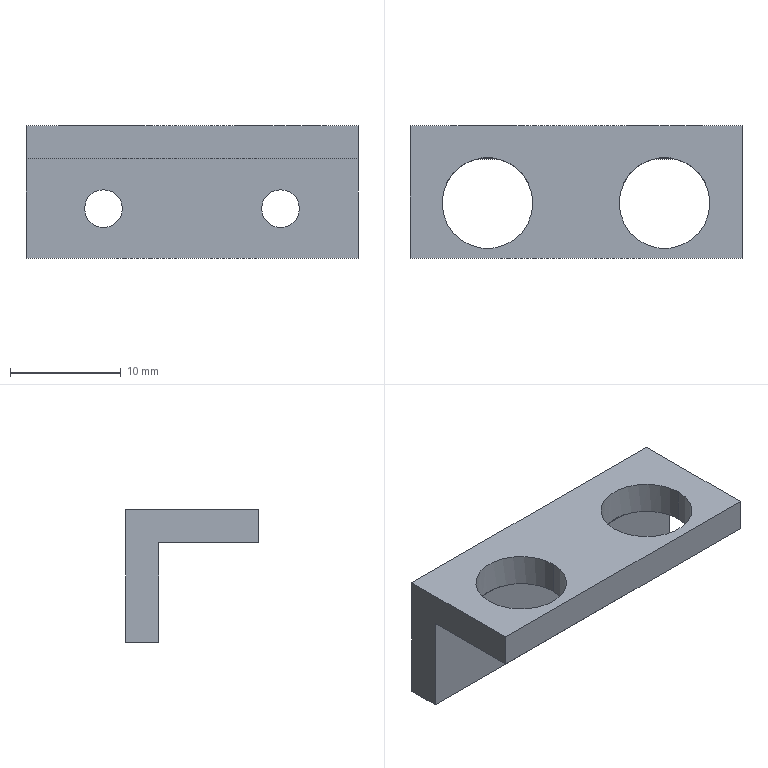NC program | NX | posted with a generic post | part box 30 x 12 x 12 mm
Lines 28 to 883 of 1871:
(ZLEVEL_PROFILE_1_1 , TOOL : D3R0.5)
N48 T07 M6
N50 G54
N52 G17 G0 G90 X-7.408 Y2.838 B0. C0. S7500 M3
N54 G43 Z30. H7
N56 Z0.929
N58 G94 G1 Z-0.071 F1000.
N60 X-7.74 Y3.413
N62 G3 X-7.999 Y3.563 R0.3
N64 X-10.062 Y1.5 R2.063 F2500.
N66 X-7.999 Y3.563 R-2.063
N68 G1 X-8.118 Y3.559 Z-0.073
N70 X-8.237 Y3.548 Z-0.075
N72 X-8.354 Y3.53 Z-0.077
N74 X-8.47 Y3.503 Z-0.079
N76 X-8.585 Y3.473 Z-0.081
N78 X-8.697 Y3.432 Z-0.083
N80 X-8.806 Y3.387 Z-0.085
N82 X-8.914 Y3.338 Z-0.087
N84 X-9.016 Y3.278 Z-0.089
N86 X-9.118 Y3.216 Z-0.092
N88 X-9.213 Y3.146 Z-0.094
N90 X-9.305 Y3.072 Z-0.096
N92 X-9.394 Y2.995 Z-0.098
N94 X-9.475 Y2.909 Z-0.1
N96 X-9.552 Y2.82 Z-0.102
N98 X-9.625 Y2.728 Z-0.104
N100 X-9.69 Y2.63 Z-0.106
N102 X-9.754 Y2.531 Z-0.108
N104 X-9.806 Y2.426 Z-0.11
N106 X-9.856 Y2.32 Z-0.112
N108 X-9.899 Y2.211 Z-0.114
N110 X-9.934 Y2.099 Z-0.116
N112 X-9.965 Y1.986 Z-0.119
N114 X-9.987 Y1.872 Z-0.121
N116 X-10.003 Y1.756 Z-0.123
N118 X-10.015 Y1.64 Z-0.125
N120 Y1.523 Z-0.127
N122 X-10.013 Y1.407 Z-0.129
N124 X-10.002 Y1.291 Z-0.131
N126 X-9.984 Y1.176 Z-0.133
N128 X-9.963 Y1.062 Z-0.135
N130 X-9.93 Y0.951 Z-0.137
N132 X-9.893 Y0.841 Z-0.139
N134 X-9.848 Y0.734 Z-0.141
N136 G3 X-7.999 Y3.501 R-2.001
N138 G1 X-8.118 Y3.497 Z-0.144
N140 X-8.237 Y3.486 Z-0.146
N142 X-8.354 Y3.467 Z-0.148
N144 X-8.47 Y3.439 Z-0.15
N146 X-8.585 Y3.409 Z-0.152
N148 X-8.696 Y3.366 Z-0.154
N150 X-8.805 Y3.321 Z-0.156
N152 X-8.912 Y3.268 Z-0.158
N154 X-9.014 Y3.208 Z-0.16
N156 X-9.114 Y3.146 Z-0.162
N158 X-9.207 Y3.073 Z-0.164
N160 X-9.298 Y2.997 Z-0.166
N162 X-9.384 Y2.916 Z-0.168
N164 X-9.464 Y2.829 Z-0.171
N166 X-9.541 Y2.741 Z-0.173
N168 X-9.609 Y2.644 Z-0.175
N170 X-9.673 Y2.546 Z-0.177
N172 X-9.731 Y2.444 Z-0.179
N174 X-9.781 Y2.338 Z-0.181
N176 X-9.828 Y2.23 Z-0.183
N178 X-9.865 Y2.119 Z-0.185
N180 X-9.897 Y2.007 Z-0.187
N182 X-9.923 Y1.893 Z-0.189
N184 X-9.94 Y1.777 Z-0.191
N186 X-9.953 Y1.661 Z-0.193
N188 X-9.955 Y1.544 Z-0.195
N190 X-9.953 Y1.428 Z-0.198
N192 X-9.944 Y1.312 Z-0.2
N194 X-9.927 Y1.197 Z-0.202
N196 X-9.904 Y1.083 Z-0.204
N198 X-9.874 Y0.971 Z-0.206
N200 X-9.837 Y0.861 Z-0.208
N202 X-9.794 Y0.754 Z-0.21
N204 X-9.744 Y0.649 Z-0.212
N206 G3 X-7.999 Y3.441 R-1.941
N208 G1 X-8.118 Y3.435 Z-0.214
N210 X-8.237 Y3.422 Z-0.216
N212 X-8.354 Y3.402 Z-0.218
N214 X-8.469 Y3.375 Z-0.22
N216 X-8.583 Y3.34 Z-0.223
N218 X-8.694 Y3.299 Z-0.225
N220 X-8.802 Y3.251 Z-0.227
N222 X-8.907 Y3.197 Z-0.229
N224 X-9.008 Y3.136 Z-0.231
N226 X-9.106 Y3.07 Z-0.233
N228 X-9.198 Y2.997 Z-0.235
N230 X-9.287 Y2.919 Z-0.237
N232 X-9.37 Y2.836 Z-0.239
N234 X-9.448 Y2.748 Z-0.241
N236 X-9.52 Y2.656 Z-0.243
N238 X-9.586 Y2.559 Z-0.245
N240 X-9.646 Y2.459 Z-0.247
N242 X-9.7 Y2.355 Z-0.25
N244 X-9.748 Y2.249 Z-0.252
N246 X-9.788 Y2.139 Z-0.254
N248 X-9.822 Y2.028 Z-0.256
N250 X-9.849 Y1.914 Z-0.258
N252 X-9.869 Y1.8 Z-0.26
N254 X-9.882 Y1.684 Z-0.262
N256 X-9.888 Y1.569 Z-0.264
N258 X-9.886 Y1.453 Z-0.266
N260 X-9.878 Y1.337 Z-0.268
N262 X-9.862 Y1.223 Z-0.27
N264 X-9.839 Y1.109 Z-0.272
N266 X-9.81 Y0.998 Z-0.275
N268 X-9.774 Y0.888 Z-0.277
N270 X-9.731 Y0.781 Z-0.279
N272 X-9.682 Y0.678 Z-0.281
N274 X-9.626 Y0.577 Z-0.283
N276 G3 X-7.999 Y3.37 R-1.87
N278 G1 X-8.118 Y3.364 Z-0.285
N280 X-8.237 Y3.351 Z-0.287
N282 X-8.353 Y3.33 Z-0.289
N284 X-8.469 Y3.302 Z-0.291
N286 X-8.582 Y3.266 Z-0.293
N288 X-8.692 Y3.224 Z-0.295
N290 X-8.8 Y3.174 Z-0.297
N292 X-8.904 Y3.118 Z-0.299
N294 X-9.004 Y3.056 Z-0.302
N296 X-9.1 Y2.987 Z-0.304
N298 X-9.191 Y2.912 Z-0.306
N300 X-9.277 Y2.832 Z-0.308
N302 X-9.357 Y2.747 Z-0.31
N304 X-9.432 Y2.656 Z-0.312
N306 X-9.501 Y2.562 Z-0.314
N308 X-9.564 Y2.463 Z-0.316
N310 X-9.621 Y2.36 Z-0.318
N312 X-9.67 Y2.254 Z-0.32
N314 X-9.713 Y2.146 Z-0.322
N316 X-9.748 Y2.035 Z-0.324
N318 X-9.777 Y1.922 Z-0.327
N320 X-9.798 Y1.808 Z-0.329
N322 X-9.812 Y1.692 Z-0.331
N324 X-9.819 Y1.576 Z-0.333
N326 X-9.818 Y1.461 Z-0.335
N328 X-9.809 Y1.345 Z-0.337
N330 X-9.794 Y1.231 Z-0.339
N332 X-9.771 Y1.117 Z-0.341
N334 X-9.741 Y1.006 Z-0.343
N336 X-9.704 Y0.897 Z-0.345
N338 X-9.66 Y0.79 Z-0.347
N340 X-9.61 Y0.687 Z-0.349
N342 X-9.553 Y0.587 Z-0.351
N344 X-9.49 Y0.491 Z-0.354
N346 G3 X-7.999 Y3.299 R-1.799
N348 G1 X-8.118 Y3.293 Z-0.356
N350 X-8.237 Y3.28 Z-0.358
N352 X-8.353 Y3.258 Z-0.36
N354 X-8.468 Y3.229 Z-0.362
N356 X-8.581 Y3.192 Z-0.364
N358 X-8.691 Y3.148 Z-0.366
N360 X-8.797 Y3.097 Z-0.368
N362 X-8.9 Y3.039 Z-0.37
N364 X-8.999 Y2.974 Z-0.372
N366 X-9.093 Y2.903 Z-0.374
N368 X-9.182 Y2.826 Z-0.376
N370 X-9.266 Y2.743 Z-0.379
N372 X-9.344 Y2.656 Z-0.381
N374 X-9.416 Y2.563 Z-0.383
N376 X-9.481 Y2.466 Z-0.385
N378 X-9.54 Y2.365 Z-0.387
N380 X-9.592 Y2.26 Z-0.389
N382 X-9.637 Y2.152 Z-0.391
N384 X-9.674 Y2.042 Z-0.393
N386 X-9.705 Y1.929 Z-0.395
N388 X-9.727 Y1.815 Z-0.397
N390 X-9.742 Y1.7 Z-0.399
N392 X-9.749 Y1.584 Z-0.401
N394 Y1.468 Z-0.403
N396 X-9.741 Y1.353 Z-0.406
N398 X-9.726 Y1.238 Z-0.408
N400 X-9.702 Y1.125 Z-0.41
N402 X-9.672 Y1.014 Z-0.412
N404 X-9.634 Y0.905 Z-0.414
N406 X-9.589 Y0.799 Z-0.416
N408 X-9.538 Y0.696 Z-0.418
N410 X-9.479 Y0.597 Z-0.42
N412 X-9.415 Y0.503 Z-0.422
N414 X-9.344 Y0.413 Z-0.424
N416 G3 X-7.999 Y3.229 R-1.729
N418 G1 X-8.118 Y3.222 Z-0.426
N420 X-8.236 Y3.208 Z-0.428
N422 X-8.353 Y3.186 Z-0.431
N424 X-8.468 Y3.155 Z-0.433
N426 X-8.58 Y3.117 Z-0.435
N428 X-8.689 Y3.072 Z-0.437
N430 X-8.795 Y3.019 Z-0.439
N432 X-8.896 Y2.959 Z-0.441
N434 X-8.993 Y2.892 Z-0.443
N436 X-9.086 Y2.818 Z-0.445
N438 X-9.172 Y2.739 Z-0.447
N440 X-9.254 Y2.654 Z-0.449
N442 X-9.328 Y2.564 Z-0.451
N444 X-9.397 Y2.468 Z-0.453
N446 X-9.458 Y2.369 Z-0.455
N448 X-9.513 Y2.265 Z-0.458
N450 X-9.56 Y2.159 Z-0.46
N452 X-9.6 Y2.049 Z-0.462
N454 X-9.632 Y1.937 Z-0.464
N456 X-9.656 Y1.823 Z-0.466
N458 X-9.672 Y1.708 Z-0.468
N460 X-9.68 Y1.592 Z-0.47
N462 X-9.681 Y1.476 Z-0.472
N464 X-9.673 Y1.361 Z-0.474
N466 X-9.657 Y1.246 Z-0.476
N468 X-9.634 Y1.133 Z-0.478
N470 X-9.603 Y1.022 Z-0.48
N472 X-9.564 Y0.913 Z-0.482
N474 X-9.518 Y0.808 Z-0.485
N476 X-9.465 Y0.706 Z-0.487
N478 X-9.405 Y0.608 Z-0.489
N480 X-9.339 Y0.515 Z-0.491
N482 X-9.266 Y0.426 Z-0.493
N484 X-9.187 Y0.343 Z-0.495
N486 G3 X-8. Y3.158 R-1.658
N488 G1 X-8.118 Y3.152 Z-0.497
N490 X-8.236 Y3.137 Z-0.499
N492 X-8.353 Y3.114 Z-0.501
N494 X-8.467 Y3.082 Z-0.503
N496 X-8.579 Y3.043 Z-0.505
N498 X-8.687 Y2.995 Z-0.507
N500 X-8.792 Y2.94 Z-0.51
N502 X-8.892 Y2.878 Z-0.512
N504 X-8.987 Y2.809 Z-0.514
N506 X-9.077 Y2.733 Z-0.516
N508 X-9.162 Y2.651 Z-0.518
N510 X-9.24 Y2.563 Z-0.52
N512 X-9.311 Y2.47 Z-0.522
N514 X-9.376 Y2.372 Z-0.524
N516 X-9.433 Y2.27 Z-0.526
N518 X-9.483 Y2.164 Z-0.528
N520 X-9.524 Y2.056 Z-0.53
N522 X-9.558 Y1.944 Z-0.532
N524 X-9.584 Y1.831 Z-0.534
N526 X-9.602 Y1.716 Z-0.537
N528 X-9.611 Y1.6 Z-0.539
N530 X-9.612 Y1.484 Z-0.541
N532 X-9.605 Y1.369 Z-0.543
N534 X-9.589 Y1.254 Z-0.545
N536 X-9.565 Y1.141 Z-0.547
N538 X-9.533 Y1.03 Z-0.549
N540 X-9.494 Y0.922 Z-0.551
N542 X-9.447 Y0.817 Z-0.553
N544 X-9.392 Y0.716 Z-0.555
N546 X-9.33 Y0.619 Z-0.557
N548 X-9.262 Y0.527 Z-0.559
N550 X-9.187 Y0.44 Z-0.562
N552 X-9.107 Y0.359 Z-0.564
N554 X-9.021 Y0.284 Z-0.566
N556 G3 X-8. Y3.087 R-1.587
N558 G1 X-8.118 Y3.081 Z-0.568
N560 X-8.236 Y3.065 Z-0.57
N562 X-8.352 Y3.041 Z-0.572
N564 X-8.467 Y3.008 Z-0.574
N566 X-8.577 Y2.967 Z-0.576
N568 X-8.685 Y2.918 Z-0.578
N570 X-8.788 Y2.861 Z-0.58
N572 X-8.887 Y2.796 Z-0.582
N574 X-8.98 Y2.724 Z-0.584
N576 X-9.068 Y2.646 Z-0.586
N578 X-9.149 Y2.561 Z-0.589
N580 X-9.224 Y2.47 Z-0.591
N582 X-9.292 Y2.375 Z-0.593
N584 X-9.352 Y2.274 Z-0.595
N586 X-9.404 Y2.17 Z-0.597
N588 X-9.449 Y2.062 Z-0.599
N590 X-9.485 Y1.951 Z-0.601
N592 X-9.512 Y1.838 Z-0.603
N594 X-9.531 Y1.724 Z-0.605
N596 X-9.542 Y1.608 Z-0.607
N598 X-9.544 Y1.492 Z-0.609
N600 X-9.536 Y1.376 Z-0.611
N602 X-9.521 Y1.262 Z-0.614
N604 X-9.497 Y1.149 Z-0.616
N606 X-9.464 Y1.038 Z-0.618
N608 X-9.423 Y0.93 Z-0.62
N610 X-9.375 Y0.826 Z-0.622
N612 X-9.319 Y0.726 Z-0.624
N614 X-9.255 Y0.631 Z-0.626
N616 X-9.185 Y0.54 Z-0.628
N618 X-9.108 Y0.456 Z-0.63
N620 X-9.025 Y0.377 Z-0.632
N622 X-8.937 Y0.305 Z-0.634
N624 X-8.843 Y0.24 Z-0.636
N626 G3 X-8. Y3.016 R-1.516
N628 G1 X-8.118 Y3.01 Z-0.638
N630 X-8.236 Y2.994 Z-0.641
N632 X-8.352 Y2.969 Z-0.643
N634 X-8.466 Y2.934 Z-0.645
N636 X-8.576 Y2.892 Z-0.647
N638 X-8.683 Y2.84 Z-0.649
N640 X-8.784 Y2.781 Z-0.651
N642 X-8.882 Y2.713 Z-0.653
N644 X-8.973 Y2.639 Z-0.655
N646 X-9.058 Y2.558 Z-0.657
N648 X-9.136 Y2.47 Z-0.659
N650 X-9.207 Y2.377 Z-0.661
N652 X-9.27 Y2.278 Z-0.663
N654 X-9.325 Y2.175 Z-0.666
N656 X-9.372 Y2.068 Z-0.668
N658 X-9.411 Y1.958 Z-0.67
N660 X-9.44 Y1.846 Z-0.672
N662 X-9.461 Y1.731 Z-0.674
N664 X-9.472 Y1.616 Z-0.676
N666 X-9.475 Y1.5 Z-0.678
N668 X-9.468 Y1.384 Z-0.68
N670 X-9.453 Y1.269 Z-0.682
N672 X-9.428 Y1.157 Z-0.684
N674 X-9.395 Y1.046 Z-0.686
N676 X-9.353 Y0.939 Z-0.688
N678 X-9.303 Y0.836 Z-0.69
N680 X-9.245 Y0.737 Z-0.693
N682 X-9.179 Y0.642 Z-0.695
N684 X-9.107 Y0.554 Z-0.697
N686 X-9.028 Y0.471 Z-0.699
N688 X-8.943 Y0.395 Z-0.701
N690 X-8.852 Y0.326 Z-0.703
N692 X-8.756 Y0.265 Z-0.705
N694 X-8.656 Y0.211 Z-0.707
N696 G3 X-8. Y2.946 R-1.446
N698 G1 X-8.118 Y2.939 Z-0.709
N700 X-8.236 Y2.922 Z-0.711
N702 X-8.352 Y2.896 Z-0.713
N704 X-8.465 Y2.86 Z-0.715
N706 X-8.574 Y2.815 Z-0.718
N708 X-8.68 Y2.762 Z-0.72
N710 X-8.78 Y2.7 Z-0.722
N712 X-8.875 Y2.63 Z-0.724
N714 X-8.964 Y2.553 Z-0.726
N716 X-9.046 Y2.468 Z-0.728
N718 X-9.12 Y2.378 Z-0.73
N720 X-9.187 Y2.281 Z-0.732
N722 X-9.245 Y2.18 Z-0.734
N724 X-9.295 Y2.074 Z-0.736
N726 X-9.336 Y1.965 Z-0.738
N728 X-9.368 Y1.853 Z-0.74
N730 X-9.39 Y1.739 Z-0.742
N732 X-9.403 Y1.623 Z-0.745
N734 X-9.406 Y1.508 Z-0.747
N736 X-9.4 Y1.392 Z-0.749
N738 X-9.384 Y1.277 Z-0.751
N740 X-9.359 Y1.165 Z-0.753
N742 X-9.325 Y1.055 Z-0.755
N744 X-9.282 Y0.948 Z-0.757
N746 X-9.23 Y0.845 Z-0.759
N748 X-9.171 Y0.747 Z-0.761
N750 X-9.103 Y0.655 Z-0.763
N752 X-9.028 Y0.568 Z-0.765
N754 X-8.947 Y0.488 Z-0.767
N756 X-8.859 Y0.415 Z-0.769
N758 X-8.765 Y0.35 Z-0.772
N760 X-8.667 Y0.293 Z-0.774
N762 X-8.565 Y0.244 Z-0.776
N764 X-8.459 Y0.204 Z-0.778
N766 G3 X-8. Y2.875 R-1.375
N768 G1 X-8.118 Y2.868 Z-0.78
N770 X-8.236 Y2.85 Z-0.782
N772 X-8.351 Y2.823 Z-0.784
N774 X-8.464 Y2.786 Z-0.786
N776 X-8.572 Y2.739 Z-0.788
N778 X-8.677 Y2.683 Z-0.79
N780 X-8.775 Y2.618 Z-0.792
N782 X-8.868 Y2.545 Z-0.794
N784 X-8.953 Y2.465 Z-0.797
N786 X-9.032 Y2.377 Z-0.799
N788 X-9.102 Y2.284 Z-0.801
N790 X-9.164 Y2.184 Z-0.803
N792 X-9.217 Y2.08 Z-0.805
N794 X-9.261 Y1.972 Z-0.807
N796 X-9.295 Y1.86 Z-0.809
N798 X-9.319 Y1.746 Z-0.811
N800 X-9.333 Y1.631 Z-0.813
N802 X-9.338 Y1.515 Z-0.815
N804 X-9.332 Y1.4 Z-0.817
N806 X-9.316 Y1.285 Z-0.819
N808 X-9.291 Y1.173 Z-0.821
N810 X-9.255 Y1.063 Z-0.824
N812 X-9.211 Y0.957 Z-0.826
N814 X-9.158 Y0.855 Z-0.828
N816 X-9.096 Y0.758 Z-0.83
N818 X-9.026 Y0.668 Z-0.832
N820 X-8.948 Y0.583 Z-0.834
N822 X-8.864 Y0.506 Z-0.836
N824 X-8.774 Y0.437 Z-0.838
N826 X-8.678 Y0.376 Z-0.84
N828 X-8.577 Y0.323 Z-0.842
N830 X-8.472 Y0.28 Z-0.844
N832 X-8.364 Y0.245 Z-0.846
N834 X-8.254 Y0.221 Z-0.849
N836 G3 X-8. Y2.804 R-1.304
N838 G1 X-8.118 Y2.797 Z-0.851
N840 X-8.236 Y2.779 Z-0.853
N842 X-8.367 Y2.745 Z-0.855
N844 X-8.463 Y2.711 Z-0.857
N846 X-8.57 Y2.662 Z-0.859
N848 X-8.673 Y2.603 Z-0.861
N850 X-8.782 Y2.525 Z-0.863
N852 X-8.859 Y2.459 Z-0.865
N854 X-8.941 Y2.376 Z-0.867
N856 X-9.016 Y2.285 Z-0.869
N858 X-9.09 Y2.173 Z-0.872
N860 X-9.138 Y2.085 Z-0.873
N862 X-9.184 Y1.978 Z-0.876
N864 X-9.221 Y1.867 Z-0.878
N866 X-9.25 Y1.738 Z-0.88
N868 X-9.263 Y1.639 Z-0.882
N870 X-9.269 Y1.523 Z-0.884
N872 X-9.264 Y1.407 Z-0.886
N874 X-9.245 Y1.277 Z-0.888
N876 X-9.222 Y1.18 Z-0.89
N878 X-9.186 Y1.071 Z-0.892
N880 X-9.14 Y0.966 Z-0.894
N882 X-9.076 Y0.851 Z-0.897
N884 X-9.02 Y0.77 Z-0.898
N886 X-8.948 Y0.681 Z-0.901
N888 X-8.868 Y0.6 Z-0.903
N890 X-8.768 Y0.516 Z-0.905
N892 X-8.687 Y0.461 Z-0.907
N894 X-8.589 Y0.404 Z-0.909
N896 X-8.485 Y0.357 Z-0.911
N898 X-8.363 Y0.315 Z-0.913
N900 X-8.269 Y0.292 Z-0.915
N902 X-8.157 Y0.274 Z-0.917
N904 X-8.045 Y0.267 Z-0.919
N906 G3 X-8. Y2.734 R-1.234
N908 G1 X-8.118 Y2.726 Z-0.921
N910 X-8.236 Y2.707 Z-0.923
N912 X-8.366 Y2.671 Z-0.926
N914 X-8.461 Y2.635 Z-0.928
N916 X-8.585 Y2.574 Z-0.93
N918 X-8.668 Y2.522 Z-0.932
N920 X-8.778 Y2.438 Z-0.934
N922 X-8.849 Y2.372 Z-0.936
N924 X-8.94 Y2.269 Z-0.938
N926 X-8.997 Y2.19 Z-0.94
N928 X-9.067 Y2.072 Z-0.942
N930 X-9.107 Y1.984 Z-0.944
N932 X-9.153 Y1.855 Z-0.947
N934 X-9.176 Y1.762 Z-0.948
N936 X-9.195 Y1.627 Z-0.951
N938 X-9.2 Y1.531 Z-0.953
N940 X-9.193 Y1.396 Z-0.955
N942 X-9.18 Y1.301 Z-0.957
N944 X-9.147 Y1.17 Z-0.959
N946 X-9.115 Y1.079 Z-0.961
N948 X-9.059 Y0.957 Z-0.963
N950 X-9.01 Y0.875 Z-0.965
N952 X-8.932 Y0.767 Z-0.967
N954 X-8.869 Y0.696 Z-0.969
N956 X-8.771 Y0.605 Z-0.972
N958 X-8.696 Y0.547 Z-0.973
N960 X-8.583 Y0.477 Z-0.976
N962 X-8.498 Y0.435 Z-0.977
N964 X-8.374 Y0.388 Z-0.98
N966 X-8.283 Y0.364 Z-0.982
N968 X-8.153 Y0.341 Z-0.984
N970 X-8.06 Y0.334 Z-0.986
N972 X-7.947 Y0.336 Z-0.988
N974 X-7.836 Y0.349 Z-0.99
N976 G3 X-8. Y2.663 R1.163
N978 G1 X-8.149 Y2.651 Z-0.993
N980 X-8.235 Y2.635 Z-0.994
N982 X-8.37 Y2.595 Z-0.997
N984 X-8.46 Y2.559 Z-0.998
N986 X-8.582 Y2.494 Z-1.001
N988 X-8.663 Y2.44 Z-1.002
N990 X-8.769 Y2.352 Z-1.005
N992 X-8.838 Y2.283 Z-1.007
N994 X-8.923 Y2.175 Z-1.009
N996 X-8.976 Y2.094 Z-1.011
N998 X-9.038 Y1.972 Z-1.013
N1000 X-9.072 Y1.881 Z-1.015
N1002 X-9.108 Y1.75 Z-1.017
N1004 X-9.123 Y1.655 Z-1.019
N1006 X-9.131 Y1.519 Z-1.021
N1008 X-9.127 Y1.423 Z-1.023
N1010 X-9.107 Y1.289 Z-1.026
N1012 X-9.084 Y1.196 Z-1.027
N1014 X-9.037 Y1.07 Z-1.03
N1016 X-8.996 Y0.984 Z-1.032
N1018 X-8.925 Y0.87 Z-1.034
N1020 X-8.867 Y0.795 Z-1.036
N1022 X-8.774 Y0.698 Z-1.038
N1024 X-8.702 Y0.637 Z-1.04
N1026 X-8.593 Y0.561 Z-1.042
N1028 X-8.51 Y0.515 Z-1.044
N1030 X-8.388 Y0.464 Z-1.046
N1032 X-8.298 Y0.436 Z-1.048
N1034 X-8.168 Y0.411 Z-1.051
N1036 X-8.075 Y0.402 Z-1.052
N1038 X-7.943 Y0.403 Z-1.055
N1040 X-7.851 Y0.414 Z-1.057
N1042 X-7.741 Y0.437 Z-1.059
N1044 X-7.634 Y0.471 Z-1.061
N1046 G3 X-8. Y2.592 R1.092
N1048 G1 X-8.15 Y2.579 Z-1.063
N1050 X-8.235 Y2.562 Z-1.065
N1052 X-8.37 Y2.521 Z-1.067
N1054 X-8.458 Y2.482 Z-1.069
N1056 X-8.578 Y2.414 Z-1.071
N1058 X-8.657 Y2.357 Z-1.073
N1060 X-8.759 Y2.264 Z-1.076
N1062 X-8.824 Y2.192 Z-1.077
N1064 X-8.903 Y2.08 Z-1.08
N1066 X-8.95 Y1.995 Z-1.081
N1068 X-9.003 Y1.869 Z-1.084
N1070 X-9.031 Y1.777 Z-1.086
N1072 X-9.055 Y1.643 Z-1.088
N1074 X-9.062 Y1.547 Z-1.09
N1076 X-9.057 Y1.411 Z-1.092
N1078 X-9.043 Y1.316 Z-1.094
N1080 X-9.009 Y1.186 Z-1.096
N1082 X-8.975 Y1.097 Z-1.098
N1084 X-8.913 Y0.977 Z-1.101
N1086 X-8.861 Y0.898 Z-1.102
N1088 X-8.775 Y0.795 Z-1.105
N1090 X-8.707 Y0.729 Z-1.106
N1092 X-8.602 Y0.647 Z-1.109
N1094 X-8.521 Y0.597 Z-1.111
N1096 X-8.401 Y0.541 Z-1.113
N1098 X-8.312 Y0.51 Z-1.115
N1100 X-8.183 Y0.481 Z-1.117
N1102 X-8.09 Y0.47 Z-1.119
N1104 X-7.959 Y0.469 Z-1.121
N1106 X-7.866 Y0.479 Z-1.123
N1108 X-7.738 Y0.507 Z-1.125
N1110 X-7.649 Y0.536 Z-1.127
N1112 X-7.548 Y0.582 Z-1.129
N1114 X-7.451 Y0.638 Z-1.131
N1116 G3 X-8. Y2.522 R1.022
N1118 G1 X-8.15 Y2.508 Z-1.134
N1120 X-8.235 Y2.49 Z-1.136
N1122 X-8.368 Y2.446 Z-1.138
N1124 X-8.455 Y2.405 Z-1.14
N1126 X-8.573 Y2.332 Z-1.142
N1128 X-8.65 Y2.272 Z-1.144
N1130 X-8.747 Y2.175 Z-1.146
N1132 X-8.807 Y2.098 Z-1.148
N1134 X-8.879 Y1.982 Z-1.15
N1136 X-8.92 Y1.894 Z-1.152
N1138 X-8.963 Y1.765 Z-1.155
N1140 X-8.982 Y1.67 Z-1.156
N1142 X-8.994 Y1.535 Z-1.159
N1144 X-8.991 Y1.439 Z-1.16
N1146 X-8.971 Y1.305 Z-1.163
N1148 X-8.946 Y1.213 Z-1.165
N1150 X-8.895 Y1.088 Z-1.167
N1152 X-8.85 Y1.004 Z-1.169
N1154 X-8.773 Y0.894 Z-1.171
N1156 X-8.709 Y0.824 Z-1.173
N1158 X-8.609 Y0.735 Z-1.175
N1160 X-8.531 Y0.682 Z-1.177
N1162 X-8.414 Y0.619 Z-1.18
N1164 X-8.326 Y0.585 Z-1.181
N1166 X-8.198 Y0.551 Z-1.184
N1168 X-8.106 Y0.538 Z-1.185
N1170 X-7.974 Y0.535 Z-1.188
N1172 X-7.881 Y0.544 Z-1.19
N1174 X-7.753 Y0.572 Z-1.192
N1176 X-7.665 Y0.601 Z-1.194
N1178 X-7.547 Y0.658 Z-1.196
N1180 X-7.468 Y0.707 Z-1.198
N1182 X-7.381 Y0.775 Z-1.2
N1184 X-7.302 Y0.854 Z-1.202
N1186 G3 X-8. Y2.451 R0.951
N1188 G1 X-8.15 Y2.436 Z-1.205
N1190 X-8.235 Y2.417 Z-1.206
N1192 X-8.367 Y2.37 Z-1.209
N1194 X-8.453 Y2.327 Z-1.21
N1196 X-8.567 Y2.25 Z-1.213
N1198 X-8.641 Y2.186 Z-1.215
N1200 X-8.732 Y2.083 Z-1.217
N1202 X-8.787 Y2.003 Z-1.219
N1204 X-8.85 Y1.882 Z-1.221
N1206 X-8.883 Y1.791 Z-1.223
N1208 X-8.914 Y1.658 Z-1.225
N1210 X-8.924 Y1.562 Z-1.227
N1212 X-8.921 Y1.427 Z-1.229
N1214 X-8.906 Y1.332 Z-1.231
N1216 X-8.87 Y1.202 Z-1.234
N1218 X-8.833 Y1.114 Z-1.235
N1220 X-8.765 Y0.998 Z-1.238
N1222 X-8.708 Y0.922 Z-1.24
N1224 X-8.614 Y0.827 Z-1.242
N1226 X-8.54 Y0.768 Z-1.244
N1228 X-8.426 Y0.7 Z-1.246
N1230 X-8.34 Y0.661 Z-1.248
N1232 X-8.213 Y0.623 Z-1.25
N1234 X-8.121 Y0.607 Z-1.252
N1236 X-7.989 Y0.602 Z-1.254
N1238 X-7.896 Y0.609 Z-1.256
N1240 X-7.768 Y0.636 Z-1.259
N1242 X-7.68 Y0.667 Z-1.26
N1244 X-7.563 Y0.725 Z-1.263
N1246 X-7.486 Y0.776 Z-1.264
N1248 X-7.387 Y0.86 Z-1.267
N1250 X-7.325 Y0.929 Z-1.269
N1252 X-7.261 Y1.018 Z-1.271
N1254 X-7.208 Y1.116 Z-1.273
N1256 G3 X-8. Y2.38 R0.88
N1258 G1 X-8.15 Y2.364 Z-1.276
N1260 X-8.234 Y2.344 Z-1.277
N1262 X-8.365 Y2.293 Z-1.28
N1264 X-8.449 Y2.247 Z-1.282
N1266 X-8.56 Y2.164 Z-1.284
N1268 X-8.629 Y2.096 Z-1.286
N1270 X-8.713 Y1.988 Z-1.289
N1272 X-8.762 Y1.904 Z-1.29
N1274 X-8.814 Y1.778 Z-1.293
N1276 X-8.838 Y1.685 Z-1.295
N1278 X-8.854 Y1.55 Z-1.297
N1280 X-8.852 Y1.454 Z-1.299
N1282 X-8.832 Y1.321 Z-1.302
N1284 X-8.805 Y1.229 Z-1.304
N1286 X-8.75 Y1.107 Z-1.306
N1288 X-8.699 Y1.026 Z-1.308
N1290 X-8.614 Y0.923 Z-1.311
N1292 X-8.544 Y0.86 Z-1.313
N1294 X-8.435 Y0.784 Z-1.315
N1296 X-8.351 Y0.741 Z-1.317
N1298 X-8.226 Y0.698 Z-1.32
N1300 X-8.134 Y0.679 Z-1.321
N1302 X-8.003 Y0.671 Z-1.324
N1304 X-7.91 Y0.678 Z-1.326
N1306 X-7.783 Y0.705 Z-1.328
N1308 X-7.695 Y0.736 Z-1.33
N1310 X-7.58 Y0.796 Z-1.333
N1312 X-7.505 Y0.849 Z-1.335
N1314 X-7.41 Y0.937 Z-1.337
N1316 X-7.352 Y1.008 Z-1.339
N1318 X-7.294 Y1.1 Z-1.341
N1320 X-7.248 Y1.201 Z-1.344
N1322 G3 X-8. Y2.309 R0.809
N1324 G1 X-8.146 Y2.293 Z-1.346
N1326 X-8.227 Y2.272 Z-1.348
N1328 X-8.354 Y2.22 Z-1.351
N1330 X-8.434 Y2.172 Z-1.353
N1332 X-8.538 Y2.088 Z-1.356
N1334 X-8.603 Y2.019 Z-1.358
N1336 X-8.678 Y1.91 Z-1.36
N1338 X-8.72 Y1.825 Z-1.362
N1340 X-8.762 Y1.7 Z-1.365
N1342 X-8.778 Y1.608 Z-1.367
N1344 X-8.783 Y1.476 Z-1.37
N1346 X-8.772 Y1.384 Z-1.372
N1348 X-8.74 Y1.258 Z-1.375
N1350 X-8.704 Y1.172 Z-1.377
N1352 X-8.637 Y1.061 Z-1.379
N1354 X-8.579 Y0.99 Z-1.381
N1356 X-8.484 Y0.902 Z-1.384
N1358 X-8.408 Y0.851 Z-1.386
N1360 X-8.293 Y0.794 Z-1.389
N1362 X-8.207 Y0.766 Z-1.391
N1364 X-8.081 Y0.745 Z-1.393
N1366 X-7.991 Y0.743 Z-1.395
N1368 X-7.865 Y0.757 Z-1.398
N1370 X-7.778 Y0.781 Z-1.4
N1372 X-7.663 Y0.83 Z-1.403
N1374 X-7.587 Y0.876 Z-1.405
N1376 X-7.49 Y0.956 Z-1.408
N1378 X-7.431 Y1.022 Z-1.41
N1380 X-7.371 Y1.109 Z-1.412
N1382 X-7.323 Y1.204 Z-1.414
N1384 G3 X-8. Y2.239 R0.739
N1386 G1 X-8.152 Y2.219 Z-1.418
N1388 X-8.236 Y2.194 Z-1.42
N1390 X-8.323 Y2.156 Z-1.422
N1392 X-8.364 Y2.133 Z-1.423
N1394 X-8.391 Y2.115 Z-1.424
N1396 X-8.444 Y2.077 Z-1.425
N1398 X-8.547 Y1.975 Z-1.428
N1400 X-8.601 Y1.901 Z-1.431
N1402 X-8.664 Y1.777 Z-1.434
N1404 X-8.693 Y1.684 Z-1.436
N1406 X-8.712 Y1.549 Z-1.439
N1408 X-8.71 Y1.452 Z-1.441
N1410 X-8.685 Y1.318 Z-1.445
N1412 X-8.651 Y1.228 Z-1.447
N1414 X-8.585 Y1.111 Z-1.45
N1416 X-8.525 Y1.036 Z-1.452
N1418 X-8.425 Y0.947 Z-1.455
N1420 X-8.345 Y0.897 Z-1.458
N1422 X-8.223 Y0.845 Z-1.461
N1424 X-8.131 Y0.823 Z-1.463
N1426 X-8. Y0.813 Z-1.466
N1428 X-7.907 Y0.822 Z-1.469
N1430 X-7.781 Y0.855 Z-1.472
N1432 X-7.696 Y0.893 Z-1.474
N1434 X-7.588 Y0.964 Z-1.477
N1436 X-7.521 Y1.027 Z-1.479
N1438 X-7.453 Y1.113 Z-1.482
N1440 X-7.399 Y1.209 Z-1.485
N1442 G3 X-8. Y2.168 R0.668
N1444 G1 X-8.099 Y2.158 Z-1.487
N1446 X-8.147 Y2.148 Z-1.489
N1448 X-8.174 Y2.14
N1450 X-8.228 Y2.122 Z-1.491
N1452 X-8.313 Y2.08 Z-1.493
N1454 X-8.354 Y2.055 Z-1.494
N1456 X-8.378 Y2.038 Z-1.495
N1458 X-8.424 Y2.001 Z-1.497
N1460 X-8.489 Y1.934 Z-1.499
N1462 X-8.518 Y1.897 Z-1.5
N1464 X-8.535 Y1.873 Z-1.501
N1466 X-8.565 Y1.822 Z-1.503
N1468 X-8.603 Y1.737 Z-1.505
N1470 X-8.617 Y1.693 Z-1.506
N1472 X-8.625 Y1.665 Z-1.507
N1474 X-8.635 Y1.607 Z-1.508
N1476 X-8.642 Y1.515 Z-1.511
N1478 X-8.64 Y1.469 Z-1.512
N1480 X-8.637 Y1.44 Z-1.513
N1482 X-8.628 Y1.383 Z-1.514
N1484 X-8.585 Y1.253 Z-1.518
N1486 X-8.544 Y1.177 Z-1.52
N1488 X-8.493 Y1.107 Z-1.523
N1490 X-8.464 Y1.075 Z-1.524
N1492 X-8.442 Y1.054 Z-1.525
N1494 X-8.396 Y1.014 Z-1.526
N1496 X-8.282 Y0.944 Z-1.53
N1498 X-8.203 Y0.913 Z-1.532
N1500 X-8.078 Y0.888 Z-1.536
N1502 X-7.989 Y0.885 Z-1.538
N1504 X-7.864 Y0.904 Z-1.541
N1506 X-7.78 Y0.932 Z-1.544
N1508 X-7.671 Y0.992 Z-1.547
N1510 X-7.602 Y1.047 Z-1.55
N1512 X-7.532 Y1.125 Z-1.553
N1514 X-7.476 Y1.214 Z-1.556
N1516 G3 X-8. Y2.097 R0.597
N1518 G1 X-8.094 Y2.087 Z-1.558
N1520 X-8.14 Y2.076 Z-1.56
N1522 X-8.166 Y2.069
N1524 X-8.218 Y2.049 Z-1.562
N1526 X-8.299 Y2.007 Z-1.565
N1528 X-8.336 Y1.981 Z-1.566
N1530 X-8.358 Y1.964 Z-1.567
N1532 X-8.401 Y1.926 Z-1.568
N1534 X-8.459 Y1.857 Z-1.571
N1536 X-8.484 Y1.82 Z-1.572
N1538 X-8.498 Y1.796 Z-1.573
N1540 X-8.523 Y1.745 Z-1.575
N1542 X-8.552 Y1.661 Z-1.578
N1544 X-8.562 Y1.618 Z-1.579
N1546 X-8.566 Y1.59 Z-1.58
N1548 X-8.571 Y1.534 Z-1.581
N1550 X-8.566 Y1.447 Z-1.584
N1552 X-8.559 Y1.404 Z-1.585
N1554 X-8.553 Y1.377 Z-1.586
N1556 X-8.537 Y1.324 Z-1.588
N1558 X-8.501 Y1.244 Z-1.59
N1560 X-8.479 Y1.207 Z-1.592
N1562 X-8.463 Y1.185 Z-1.593
N1564 X-8.429 Y1.142 Z-1.594
N1566 X-8.367 Y1.082 Z-1.597
N1568 X-8.333 Y1.057 Z-1.598
N1570 X-8.311 Y1.042 Z-1.599
N1572 X-8.264 Y1.015 Z-1.601
N1574 X-8.185 Y0.982 Z-1.603
N1576 X-8.145 Y0.971 Z-1.605
N1578 X-8.119 Y0.966
N1580 X-8.066 Y0.958 Z-1.607
N1582 X-7.982 Y0.957 Z-1.61
N1584 X-7.94 Y0.961 Z-1.611
N1586 X-7.914 Y0.966 Z-1.612
N1588 X-7.863 Y0.978 Z-1.613
N1590 X-7.749 Y1.027 Z-1.617
N1592 X-7.684 Y1.071 Z-1.62
N1594 X-7.612 Y1.14 Z-1.623
N1596 X-7.553 Y1.221 Z-1.626
N1598 G3 X-8. Y2.027 R0.527
N1600 G1 X-8.1 Y2.014 Z-1.63
N1602 X-8.148 Y2. Z-1.631
N1604 X-8.175 Y1.99 Z-1.632
N1606 X-8.227 Y1.966 Z-1.634
N1608 X-8.308 Y1.914 Z-1.637
N1610 X-8.343 Y1.883 Z-1.639
N1612 X-8.364 Y1.861 Z-1.64
N1614 X-8.402 Y1.815 Z-1.642
N1616 X-8.451 Y1.734 Z-1.645
N1618 X-8.469 Y1.691 Z-1.647
N1620 X-8.478 Y1.663 Z-1.648
N1622 X-8.492 Y1.605 Z-1.65
N1624 X-8.5 Y1.513 Z-1.653
N1626 X-8.497 Y1.467 Z-1.655
N1628 X-8.493 Y1.438 Z-1.656
N1630 X-8.481 Y1.381 Z-1.658
N1632 X-8.448 Y1.296 Z-1.661
N1634 X-8.426 Y1.257 Z-1.663
N1636 X-8.41 Y1.233 Z-1.664
N1638 X-8.374 Y1.188 Z-1.666
N1640 X-8.308 Y1.127 Z-1.669
N1642 X-8.272 Y1.101 Z-1.67
N1644 X-8.248 Y1.087 Z-1.671
N1646 X-8.196 Y1.063 Z-1.673
N1648 X-8.112 Y1.037 Z-1.677
N1650 X-8.069 Y1.03 Z-1.678
N1652 X-8.041 Y1.028 Z-1.679
N1654 X-7.985 Y1.029 Z-1.681
N1656 X-7.899 Y1.043 Z-1.685
N1658 X-7.859 Y1.055 Z-1.686
N1660 X-7.833 Y1.065 Z-1.687
N1662 X-7.784 Y1.09 Z-1.689
N1664 X-7.74 Y1.118 Z-1.691
N1666 X-7.701 Y1.151 Z-1.693
N1668 X-7.665 Y1.188 Z-1.695
N1670 X-7.633 Y1.23 Z-1.697
N1672 G3 X-8. Y1.956 R0.456
N1674 G1 X-8.094 Y1.942 Z-1.701
N1676 X-8.139 Y1.928 Z-1.703
N1678 X-8.164 Y1.918 Z-1.704
N1680 X-8.213 Y1.893 Z-1.706
N1682 X-8.286 Y1.839 Z-1.709
N1684 X-8.317 Y1.807 Z-1.711
N1686 X-8.336 Y1.785 Z-1.712
N1688 X-8.368 Y1.739 Z-1.715
N1690 X-8.405 Y1.658 Z-1.718
N1692 X-8.417 Y1.616 Z-1.72
N1694 X-8.422 Y1.589 Z-1.721
N1696 X-8.428 Y1.533 Z-1.724
N1698 X-8.422 Y1.447 Z-1.727
N1700 X-8.413 Y1.405 Z-1.729
N1702 X-8.405 Y1.379 Z-1.73
N1704 X-8.384 Y1.329 Z-1.732
N1706 X-8.339 Y1.257 Z-1.736
N1708 X-8.311 Y1.225 Z-1.738
N1710 X-8.292 Y1.207 Z-1.739
N1712 X-8.25 Y1.173 Z-1.741
N1714 X-8.178 Y1.133 Z-1.745
N1716 X-8.139 Y1.118 Z-1.747
N1718 X-8.114 Y1.111 Z-1.748
N1720 X-8.063 Y1.102 Z-1.75
N1722 X-7.981 Y1.101 Z-1.754
N1724 X-7.942 Y1.107 Z-1.755
N1726 X-7.917 Y1.113 Z-1.757
N1728 X-7.868 Y1.129 Z-1.759
N1730 X-7.824 Y1.15 Z-1.761
N1732 X-7.784 Y1.176 Z-1.763
N1734 X-7.747 Y1.207 Z-1.766
N1736 X-7.713 Y1.243 Z-1.768
N1738 G3 X-8. Y1.885 R0.385
N1740 G1 X-8.1 Y1.867 Z-1.773
N1742 X-8.146 Y1.848 Z-1.775
N1744 X-8.22 Y1.802 Z-1.78
N1746 X-8.284 Y1.733 Z-1.784
N1748 X-8.307 Y1.695 Z-1.787
N1750 X-8.321 Y1.667 Z-1.788
N1752 X-8.344 Y1.61 Z-1.791